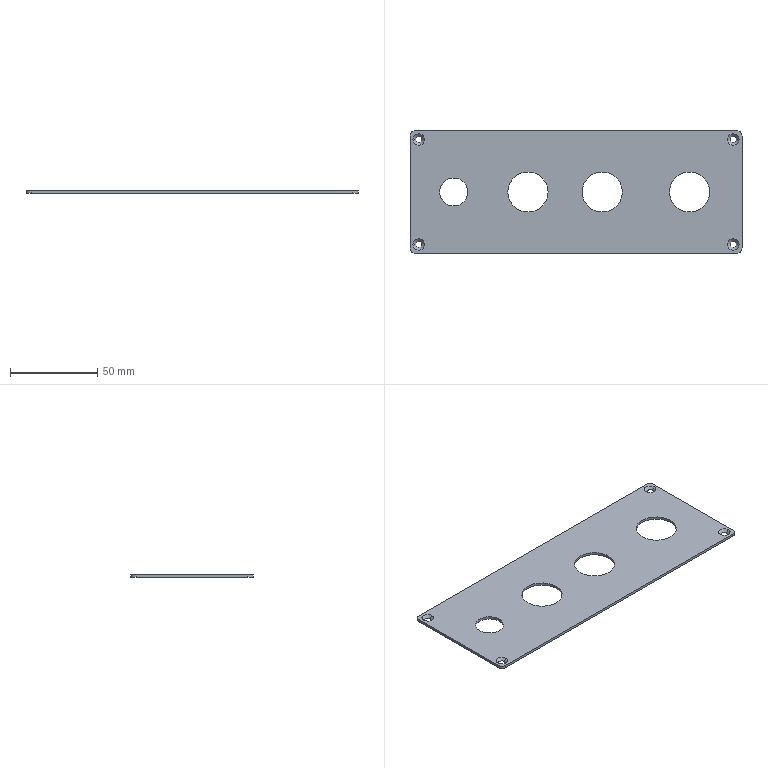Part | SolidWorks | features Extrusion 1, Fillet 1, HoleWzd 1, ICE 1 | 1 solid | 26 faces | box 190 x 70 x 1.5 mm | volume 17641 mm3 | cylinder 12 | cone 8 | plane 6 | commonest cylinder face diameters 23 x6 6 x4 16 x2
STEP:
#1=CARTESIAN_POINT('',(-91.8,30.,0.));
#2=VERTEX_POINT('',#1);
#3=CARTESIAN_POINT('',(-88.2,30.,0.));
#4=VERTEX_POINT('',#3);
#5=CARTESIAN_POINT('',(-90.,30.,0.));
#6=DIRECTION('',(0.,0.,1.));
#7=DIRECTION('',(1.,0.,0.));
#8=AXIS2_PLACEMENT_3D('',#5,#6,#7);
#9=CIRCLE('',#8,1.8);
#10=EDGE_CURVE('',#2,#4,#9,.T.);
#11=ORIENTED_EDGE('',*,*,#10,.F.);
#12=CARTESIAN_POINT('',(-93.3,30.,1.5));
#13=VERTEX_POINT('',#12);
#14=CARTESIAN_POINT('',(-93.3,30.,1.5));
#15=DIRECTION('',(-0.7071,0.,0.7071));
#16=VECTOR('',#15,1000.);
#17=LINE('',#14,#16);
#18=EDGE_CURVE('',#2,#13,#17,.T.);
#19=ORIENTED_EDGE('',*,*,#18,.T.);
#20=CARTESIAN_POINT('',(-86.7,30.,1.5));
#21=VERTEX_POINT('',#20);
#22=CARTESIAN_POINT('',(-90.,30.,1.5));
#23=DIRECTION('',(0.,0.,1.));
#24=DIRECTION('',(1.,0.,0.));
#25=AXIS2_PLACEMENT_3D('',#22,#23,#24);
#26=CIRCLE('',#25,3.3);
#27=EDGE_CURVE('',#13,#21,#26,.T.);
#28=ORIENTED_EDGE('',*,*,#27,.T.);
#29=CARTESIAN_POINT('',(-86.7,30.,1.5));
#30=DIRECTION('',(0.7071,0.,0.7071));
#31=VECTOR('',#30,1000.);
#32=LINE('',#29,#31);
#33=EDGE_CURVE('',#4,#21,#32,.T.);
#34=ORIENTED_EDGE('',*,*,#33,.F.);
#35=EDGE_LOOP('',(#11,#19,#28,#34));
#36=FACE_OUTER_BOUND('',#35,.T.);
#37=CARTESIAN_POINT('',(-90.,30.,1.5));
#38=DIRECTION('',(0.,0.,1.));
#39=DIRECTION('',(1.,0.,0.));
#40=AXIS2_PLACEMENT_3D('',#37,#38,#39);
#41=CONICAL_SURFACE('',#40,3.3,0.7854);
#42=ADVANCED_FACE('',(#36),#41,.F.);
#43=CARTESIAN_POINT('',(-91.8,-30.,0.));
#44=VERTEX_POINT('',#43);
#45=CARTESIAN_POINT('',(-88.2,-30.,0.));
#46=VERTEX_POINT('',#45);
#47=CARTESIAN_POINT('',(-90.,-30.,0.));
#48=DIRECTION('',(0.,0.,1.));
#49=DIRECTION('',(1.,0.,0.));
#50=AXIS2_PLACEMENT_3D('',#47,#48,#49);
#51=CIRCLE('',#50,1.8);
#52=EDGE_CURVE('',#44,#46,#51,.T.);
#53=ORIENTED_EDGE('',*,*,#52,.F.);
#54=CARTESIAN_POINT('',(-93.3,-30.,1.5));
#55=VERTEX_POINT('',#54);
#56=CARTESIAN_POINT('',(-93.3,-30.,1.5));
#57=DIRECTION('',(-0.7071,0.,0.7071));
#58=VECTOR('',#57,1000.);
#59=LINE('',#56,#58);
#60=EDGE_CURVE('',#44,#55,#59,.T.);
#61=ORIENTED_EDGE('',*,*,#60,.T.);
#62=CARTESIAN_POINT('',(-86.7,-30.,1.5));
#63=VERTEX_POINT('',#62);
#64=CARTESIAN_POINT('',(-90.,-30.,1.5));
#65=DIRECTION('',(0.,0.,1.));
#66=DIRECTION('',(1.,0.,0.));
#67=AXIS2_PLACEMENT_3D('',#64,#65,#66);
#68=CIRCLE('',#67,3.3);
#69=EDGE_CURVE('',#55,#63,#68,.T.);
#70=ORIENTED_EDGE('',*,*,#69,.T.);
#71=CARTESIAN_POINT('',(-86.7,-30.,1.5));
#72=DIRECTION('',(0.7071,0.,0.7071));
#73=VECTOR('',#72,1000.);
#74=LINE('',#71,#73);
#75=EDGE_CURVE('',#46,#63,#74,.T.);
#76=ORIENTED_EDGE('',*,*,#75,.F.);
#77=EDGE_LOOP('',(#53,#61,#70,#76));
#78=FACE_OUTER_BOUND('',#77,.T.);
#79=CARTESIAN_POINT('',(-90.,-30.,1.5));
#80=DIRECTION('',(0.,0.,1.));
#81=DIRECTION('',(1.,0.,0.));
#82=AXIS2_PLACEMENT_3D('',#79,#80,#81);
#83=CONICAL_SURFACE('',#82,3.3,0.7854);
#84=ADVANCED_FACE('',(#78),#83,.F.);
#85=CARTESIAN_POINT('',(88.2,-30.,0.));
#86=VERTEX_POINT('',#85);
#87=CARTESIAN_POINT('',(91.8,-30.,0.));
#88=VERTEX_POINT('',#87);
#89=CARTESIAN_POINT('',(90.,-30.,0.));
#90=DIRECTION('',(0.,0.,1.));
#91=DIRECTION('',(1.,0.,0.));
#92=AXIS2_PLACEMENT_3D('',#89,#90,#91);
#93=CIRCLE('',#92,1.8);
#94=EDGE_CURVE('',#86,#88,#93,.T.);
#95=ORIENTED_EDGE('',*,*,#94,.F.);
#96=CARTESIAN_POINT('',(86.7,-30.,1.5));
#97=VERTEX_POINT('',#96);
#98=CARTESIAN_POINT('',(86.7,-30.,1.5));
#99=DIRECTION('',(-0.7071,0.,0.7071));
#100=VECTOR('',#99,1000.);
#101=LINE('',#98,#100);
#102=EDGE_CURVE('',#86,#97,#101,.T.);
#103=ORIENTED_EDGE('',*,*,#102,.T.);
#104=CARTESIAN_POINT('',(93.3,-30.,1.5));
#105=VERTEX_POINT('',#104);
#106=CARTESIAN_POINT('',(90.,-30.,1.5));
#107=DIRECTION('',(0.,0.,1.));
#108=DIRECTION('',(1.,0.,0.));
#109=AXIS2_PLACEMENT_3D('',#106,#107,#108);
#110=CIRCLE('',#109,3.3);
#111=EDGE_CURVE('',#97,#105,#110,.T.);
#112=ORIENTED_EDGE('',*,*,#111,.T.);
#113=CARTESIAN_POINT('',(93.3,-30.,1.5));
#114=DIRECTION('',(0.7071,0.,0.7071));
#115=VECTOR('',#114,1000.);
#116=LINE('',#113,#115);
#117=EDGE_CURVE('',#88,#105,#116,.T.);
#118=ORIENTED_EDGE('',*,*,#117,.F.);
#119=EDGE_LOOP('',(#95,#103,#112,#118));
#120=FACE_OUTER_BOUND('',#119,.T.);
#121=CARTESIAN_POINT('',(90.,-30.,1.5));
#122=DIRECTION('',(0.,0.,1.));
#123=DIRECTION('',(1.,0.,0.));
#124=AXIS2_PLACEMENT_3D('',#121,#122,#123);
#125=CONICAL_SURFACE('',#124,3.3,0.7854);
#126=ADVANCED_FACE('',(#120),#125,.F.);
#127=CARTESIAN_POINT('',(88.2,30.,0.));
#128=VERTEX_POINT('',#127);
#129=CARTESIAN_POINT('',(91.8,30.,0.));
#130=VERTEX_POINT('',#129);
#131=CARTESIAN_POINT('',(90.,30.,0.));
#132=DIRECTION('',(0.,0.,1.));
#133=DIRECTION('',(1.,0.,0.));
#134=AXIS2_PLACEMENT_3D('',#131,#132,#133);
#135=CIRCLE('',#134,1.8);
#136=EDGE_CURVE('',#128,#130,#135,.T.);
#137=ORIENTED_EDGE('',*,*,#136,.F.);
#138=CARTESIAN_POINT('',(86.7,30.,1.5));
#139=VERTEX_POINT('',#138);
#140=CARTESIAN_POINT('',(86.7,30.,1.5));
#141=DIRECTION('',(-0.7071,0.,0.7071));
#142=VECTOR('',#141,1000.);
#143=LINE('',#140,#142);
#144=EDGE_CURVE('',#128,#139,#143,.T.);
#145=ORIENTED_EDGE('',*,*,#144,.T.);
#146=CARTESIAN_POINT('',(93.3,30.,1.5));
#147=VERTEX_POINT('',#146);
#148=CARTESIAN_POINT('',(90.,30.,1.5));
#149=DIRECTION('',(0.,0.,1.));
#150=DIRECTION('',(1.,0.,0.));
#151=AXIS2_PLACEMENT_3D('',#148,#149,#150);
#152=CIRCLE('',#151,3.3);
#153=EDGE_CURVE('',#139,#147,#152,.T.);
#154=ORIENTED_EDGE('',*,*,#153,.T.);
#155=CARTESIAN_POINT('',(93.3,30.,1.5));
#156=DIRECTION('',(0.7071,0.,0.7071));
#157=VECTOR('',#156,1000.);
#158=LINE('',#155,#157);
#159=EDGE_CURVE('',#130,#147,#158,.T.);
#160=ORIENTED_EDGE('',*,*,#159,.F.);
#161=EDGE_LOOP('',(#137,#145,#154,#160));
#162=FACE_OUTER_BOUND('',#161,.T.);
#163=CARTESIAN_POINT('',(90.,30.,1.5));
#164=DIRECTION('',(0.,0.,1.));
#165=DIRECTION('',(1.,0.,0.));
#166=AXIS2_PLACEMENT_3D('',#163,#164,#165);
#167=CONICAL_SURFACE('',#166,3.3,0.7854);
#168=ADVANCED_FACE('',(#162),#167,.F.);
#169=CARTESIAN_POINT('',(53.5,0.,0.));
#170=VERTEX_POINT('',#169);
#171=CARTESIAN_POINT('',(76.5,0.,0.));
#172=VERTEX_POINT('',#171);
#173=CARTESIAN_POINT('',(65.,0.,0.));
#174=DIRECTION('',(0.,0.,1.));
#175=DIRECTION('',(1.,0.,0.));
#176=AXIS2_PLACEMENT_3D('',#173,#174,#175);
#177=CIRCLE('',#176,11.5);
#178=EDGE_CURVE('',#170,#172,#177,.T.);
#179=ORIENTED_EDGE('',*,*,#178,.F.);
#180=CARTESIAN_POINT('',(53.5,0.,1.5));
#181=VERTEX_POINT('',#180);
#182=CARTESIAN_POINT('',(53.5,0.,0.));
#183=DIRECTION('',(0.,0.,1.));
#184=VECTOR('',#183,1000.);
#185=LINE('',#182,#184);
#186=EDGE_CURVE('',#170,#181,#185,.T.);
#187=ORIENTED_EDGE('',*,*,#186,.T.);
#188=CARTESIAN_POINT('',(76.5,0.,1.5));
#189=VERTEX_POINT('',#188);
#190=CARTESIAN_POINT('',(65.,0.,1.5));
#191=DIRECTION('',(0.,0.,1.));
#192=DIRECTION('',(1.,0.,0.));
#193=AXIS2_PLACEMENT_3D('',#190,#191,#192);
#194=CIRCLE('',#193,11.5);
#195=EDGE_CURVE('',#181,#189,#194,.T.);
#196=ORIENTED_EDGE('',*,*,#195,.T.);
#197=CARTESIAN_POINT('',(76.5,0.,0.));
#198=DIRECTION('',(0.,0.,1.));
#199=VECTOR('',#198,1000.);
#200=LINE('',#197,#199);
#201=EDGE_CURVE('',#172,#189,#200,.T.);
#202=ORIENTED_EDGE('',*,*,#201,.F.);
#203=EDGE_LOOP('',(#179,#187,#196,#202));
#204=FACE_OUTER_BOUND('',#203,.T.);
#205=CARTESIAN_POINT('',(65.,0.,0.));
#206=DIRECTION('',(0.,0.,1.));
#207=DIRECTION('',(1.,0.,0.));
#208=AXIS2_PLACEMENT_3D('',#205,#206,#207);
#209=CYLINDRICAL_SURFACE('',#208,11.5);
#210=ADVANCED_FACE('',(#204),#209,.F.);
#211=CARTESIAN_POINT('',(-78.,0.,0.));
#212=VERTEX_POINT('',#211);
#213=CARTESIAN_POINT('',(-62.,0.,0.));
#214=VERTEX_POINT('',#213);
#215=CARTESIAN_POINT('',(-70.,0.,0.));
#216=DIRECTION('',(0.,0.,1.));
#217=DIRECTION('',(1.,0.,0.));
#218=AXIS2_PLACEMENT_3D('',#215,#216,#217);
#219=CIRCLE('',#218,8.);
#220=EDGE_CURVE('',#212,#214,#219,.T.);
#221=ORIENTED_EDGE('',*,*,#220,.F.);
#222=CARTESIAN_POINT('',(-78.,0.,1.5));
#223=VERTEX_POINT('',#222);
#224=CARTESIAN_POINT('',(-78.,0.,0.));
#225=DIRECTION('',(0.,0.,1.));
#226=VECTOR('',#225,1000.);
#227=LINE('',#224,#226);
#228=EDGE_CURVE('',#212,#223,#227,.T.);
#229=ORIENTED_EDGE('',*,*,#228,.T.);
#230=CARTESIAN_POINT('',(-62.,0.,1.5));
#231=VERTEX_POINT('',#230);
#232=CARTESIAN_POINT('',(-70.,0.,1.5));
#233=DIRECTION('',(0.,0.,1.));
#234=DIRECTION('',(1.,0.,0.));
#235=AXIS2_PLACEMENT_3D('',#232,#233,#234);
#236=CIRCLE('',#235,8.);
#237=EDGE_CURVE('',#223,#231,#236,.T.);
#238=ORIENTED_EDGE('',*,*,#237,.T.);
#239=CARTESIAN_POINT('',(-62.,0.,0.));
#240=DIRECTION('',(0.,0.,1.));
#241=VECTOR('',#240,1000.);
#242=LINE('',#239,#241);
#243=EDGE_CURVE('',#214,#231,#242,.T.);
#244=ORIENTED_EDGE('',*,*,#243,.F.);
#245=EDGE_LOOP('',(#221,#229,#238,#244));
#246=FACE_OUTER_BOUND('',#245,.T.);
#247=CARTESIAN_POINT('',(-70.,0.,0.));
#248=DIRECTION('',(0.,0.,1.));
#249=DIRECTION('',(1.,0.,0.));
#250=AXIS2_PLACEMENT_3D('',#247,#248,#249);
#251=CYLINDRICAL_SURFACE('',#250,8.);
#252=ADVANCED_FACE('',(#246),#251,.F.);
#253=CARTESIAN_POINT('',(-39.,0.,0.));
#254=VERTEX_POINT('',#253);
#255=CARTESIAN_POINT('',(-16.,0.,0.));
#256=VERTEX_POINT('',#255);
#257=CARTESIAN_POINT('',(-27.5,0.,0.));
#258=DIRECTION('',(0.,0.,1.));
#259=DIRECTION('',(1.,0.,0.));
#260=AXIS2_PLACEMENT_3D('',#257,#258,#259);
#261=CIRCLE('',#260,11.5);
#262=EDGE_CURVE('',#254,#256,#261,.T.);
#263=ORIENTED_EDGE('',*,*,#262,.F.);
#264=CARTESIAN_POINT('',(-39.,0.,1.5));
#265=VERTEX_POINT('',#264);
#266=CARTESIAN_POINT('',(-39.,0.,0.));
#267=DIRECTION('',(0.,0.,1.));
#268=VECTOR('',#267,1000.);
#269=LINE('',#266,#268);
#270=EDGE_CURVE('',#254,#265,#269,.T.);
#271=ORIENTED_EDGE('',*,*,#270,.T.);
#272=CARTESIAN_POINT('',(-16.,0.,1.5));
#273=VERTEX_POINT('',#272);
#274=CARTESIAN_POINT('',(-27.5,0.,1.5));
#275=DIRECTION('',(0.,0.,1.));
#276=DIRECTION('',(1.,0.,0.));
#277=AXIS2_PLACEMENT_3D('',#274,#275,#276);
#278=CIRCLE('',#277,11.5);
#279=EDGE_CURVE('',#265,#273,#278,.T.);
#280=ORIENTED_EDGE('',*,*,#279,.T.);
#281=CARTESIAN_POINT('',(-16.,0.,0.));
#282=DIRECTION('',(0.,0.,1.));
#283=VECTOR('',#282,1000.);
#284=LINE('',#281,#283);
#285=EDGE_CURVE('',#256,#273,#284,.T.);
#286=ORIENTED_EDGE('',*,*,#285,.F.);
#287=EDGE_LOOP('',(#263,#271,#280,#286));
#288=FACE_OUTER_BOUND('',#287,.T.);
#289=CARTESIAN_POINT('',(-27.5,0.,0.));
#290=DIRECTION('',(0.,0.,1.));
#291=DIRECTION('',(1.,0.,0.));
#292=AXIS2_PLACEMENT_3D('',#289,#290,#291);
#293=CYLINDRICAL_SURFACE('',#292,11.5);
#294=ADVANCED_FACE('',(#288),#293,.F.);
#295=CARTESIAN_POINT('',(3.5,0.,0.));
#296=VERTEX_POINT('',#295);
#297=CARTESIAN_POINT('',(26.5,0.,0.));
#298=VERTEX_POINT('',#297);
#299=CARTESIAN_POINT('',(15.,0.,0.));
#300=DIRECTION('',(0.,0.,1.));
#301=DIRECTION('',(1.,0.,0.));
#302=AXIS2_PLACEMENT_3D('',#299,#300,#301);
#303=CIRCLE('',#302,11.5);
#304=EDGE_CURVE('',#296,#298,#303,.T.);
#305=ORIENTED_EDGE('',*,*,#304,.F.);
#306=CARTESIAN_POINT('',(3.5,0.,1.5));
#307=VERTEX_POINT('',#306);
#308=CARTESIAN_POINT('',(3.5,0.,0.));
#309=DIRECTION('',(0.,0.,1.));
#310=VECTOR('',#309,1000.);
#311=LINE('',#308,#310);
#312=EDGE_CURVE('',#296,#307,#311,.T.);
#313=ORIENTED_EDGE('',*,*,#312,.T.);
#314=CARTESIAN_POINT('',(26.5,0.,1.5));
#315=VERTEX_POINT('',#314);
#316=CARTESIAN_POINT('',(15.,0.,1.5));
#317=DIRECTION('',(0.,0.,1.));
#318=DIRECTION('',(1.,0.,0.));
#319=AXIS2_PLACEMENT_3D('',#316,#317,#318);
#320=CIRCLE('',#319,11.5);
#321=EDGE_CURVE('',#307,#315,#320,.T.);
#322=ORIENTED_EDGE('',*,*,#321,.T.);
#323=CARTESIAN_POINT('',(26.5,0.,0.));
#324=DIRECTION('',(0.,0.,1.));
#325=VECTOR('',#324,1000.);
#326=LINE('',#323,#325);
#327=EDGE_CURVE('',#298,#315,#326,.T.);
#328=ORIENTED_EDGE('',*,*,#327,.F.);
#329=EDGE_LOOP('',(#305,#313,#322,#328));
#330=FACE_OUTER_BOUND('',#329,.T.);
#331=CARTESIAN_POINT('',(15.,0.,0.));
#332=DIRECTION('',(0.,0.,1.));
#333=DIRECTION('',(1.,0.,0.));
#334=AXIS2_PLACEMENT_3D('',#331,#332,#333);
#335=CYLINDRICAL_SURFACE('',#334,11.5);
#336=ADVANCED_FACE('',(#330),#335,.F.);
#337=CARTESIAN_POINT('',(-90.,30.,0.));
#338=DIRECTION('',(0.,0.,1.));
#339=DIRECTION('',(1.,0.,0.));
#340=AXIS2_PLACEMENT_3D('',#337,#338,#339);
#341=CIRCLE('',#340,1.8);
#342=EDGE_CURVE('',#4,#2,#341,.T.);
#343=ORIENTED_EDGE('',*,*,#342,.T.);
#344=ORIENTED_EDGE('',*,*,#10,.T.);
#345=EDGE_LOOP('',(#343,#344));
#346=FACE_BOUND('',#345,.T.);
#347=CARTESIAN_POINT('',(-90.,-30.,0.));
#348=DIRECTION('',(0.,0.,1.));
#349=DIRECTION('',(1.,0.,0.));
#350=AXIS2_PLACEMENT_3D('',#347,#348,#349);
#351=CIRCLE('',#350,1.8);
#352=EDGE_CURVE('',#46,#44,#351,.T.);
#353=ORIENTED_EDGE('',*,*,#352,.T.);
#354=ORIENTED_EDGE('',*,*,#52,.T.);
#355=EDGE_LOOP('',(#353,#354));
#356=FACE_BOUND('',#355,.T.);
#357=CARTESIAN_POINT('',(90.,-30.,0.));
#358=DIRECTION('',(0.,0.,1.));
#359=DIRECTION('',(1.,0.,0.));
#360=AXIS2_PLACEMENT_3D('',#357,#358,#359);
#361=CIRCLE('',#360,1.8);
#362=EDGE_CURVE('',#88,#86,#361,.T.);
#363=ORIENTED_EDGE('',*,*,#362,.T.);
#364=ORIENTED_EDGE('',*,*,#94,.T.);
#365=EDGE_LOOP('',(#363,#364));
#366=FACE_BOUND('',#365,.T.);
#367=CARTESIAN_POINT('',(90.,30.,0.));
#368=DIRECTION('',(0.,0.,1.));
#369=DIRECTION('',(1.,0.,0.));
#370=AXIS2_PLACEMENT_3D('',#367,#368,#369);
#371=CIRCLE('',#370,1.8);
#372=EDGE_CURVE('',#130,#128,#371,.T.);
#373=ORIENTED_EDGE('',*,*,#372,.T.);
#374=ORIENTED_EDGE('',*,*,#136,.T.);
#375=EDGE_LOOP('',(#373,#374));
#376=FACE_BOUND('',#375,.T.);
#377=CARTESIAN_POINT('',(65.,0.,0.));
#378=DIRECTION('',(0.,0.,1.));
#379=DIRECTION('',(1.,0.,0.));
#380=AXIS2_PLACEMENT_3D('',#377,#378,#379);
#381=CIRCLE('',#380,11.5);
#382=EDGE_CURVE('',#172,#170,#381,.T.);
#383=ORIENTED_EDGE('',*,*,#382,.T.);
#384=ORIENTED_EDGE('',*,*,#178,.T.);
#385=EDGE_LOOP('',(#383,#384));
#386=FACE_BOUND('',#385,.T.);
#387=CARTESIAN_POINT('',(-70.,0.,0.));
#388=DIRECTION('',(0.,0.,1.));
#389=DIRECTION('',(1.,0.,0.));
#390=AXIS2_PLACEMENT_3D('',#387,#388,#389);
#391=CIRCLE('',#390,8.);
#392=EDGE_CURVE('',#214,#212,#391,.T.);
#393=ORIENTED_EDGE('',*,*,#392,.T.);
#394=ORIENTED_EDGE('',*,*,#220,.T.);
#395=EDGE_LOOP('',(#393,#394));
#396=FACE_BOUND('',#395,.T.);
#397=CARTESIAN_POINT('',(-27.5,0.,0.));
#398=DIRECTION('',(0.,0.,1.));
#399=DIRECTION('',(1.,0.,0.));
#400=AXIS2_PLACEMENT_3D('',#397,#398,#399);
#401=CIRCLE('',#400,11.5);
#402=EDGE_CURVE('',#256,#254,#401,.T.);
#403=ORIENTED_EDGE('',*,*,#402,.T.);
#404=ORIENTED_EDGE('',*,*,#262,.T.);
#405=EDGE_LOOP('',(#403,#404));
#406=FACE_BOUND('',#405,.T.);
#407=CARTESIAN_POINT('',(15.,0.,0.));
#408=DIRECTION('',(0.,0.,1.));
#409=DIRECTION('',(1.,0.,0.));
#410=AXIS2_PLACEMENT_3D('',#407,#408,#409);
#411=CIRCLE('',#410,11.5);
#412=EDGE_CURVE('',#298,#296,#411,.T.);
#413=ORIENTED_EDGE('',*,*,#412,.T.);
#414=ORIENTED_EDGE('',*,*,#304,.T.);
#415=EDGE_LOOP('',(#413,#414));
#416=FACE_BOUND('',#415,.T.);
#417=CARTESIAN_POINT('',(-95.,32.,0.));
#418=VERTEX_POINT('',#417);
#419=CARTESIAN_POINT('',(-95.,-32.,0.));
#420=VERTEX_POINT('',#419);
#421=CARTESIAN_POINT('',(-95.,35.,0.));
#422=DIRECTION('',(0.,-1.,0.));
#423=VECTOR('',#422,1000.);
#424=LINE('',#421,#423);
#425=EDGE_CURVE('',#418,#420,#424,.T.);
#426=ORIENTED_EDGE('',*,*,#425,.F.);
#427=CARTESIAN_POINT('',(-92.,35.,0.));
#428=VERTEX_POINT('',#427);
#429=CARTESIAN_POINT('',(-92.,32.,0.));
#430=DIRECTION('',(0.,0.,-1.));
#431=DIRECTION('',(1.,0.,0.));
#432=AXIS2_PLACEMENT_3D('',#429,#430,#431);
#433=CIRCLE('',#432,3.);
#434=EDGE_CURVE('',#418,#428,#433,.T.);
#435=ORIENTED_EDGE('',*,*,#434,.T.);
#436=CARTESIAN_POINT('',(92.,35.,0.));
#437=VERTEX_POINT('',#436);
#438=CARTESIAN_POINT('',(-95.,35.,0.));
#439=DIRECTION('',(-1.,0.,0.));
#440=VECTOR('',#439,1000.);
#441=LINE('',#438,#440);
#442=EDGE_CURVE('',#437,#428,#441,.T.);
#443=ORIENTED_EDGE('',*,*,#442,.F.);
#444=CARTESIAN_POINT('',(95.,32.,0.));
#445=VERTEX_POINT('',#444);
#446=CARTESIAN_POINT('',(92.,32.,0.));
#447=DIRECTION('',(0.,0.,-1.));
#448=DIRECTION('',(1.,0.,0.));
#449=AXIS2_PLACEMENT_3D('',#446,#447,#448);
#450=CIRCLE('',#449,3.);
#451=EDGE_CURVE('',#437,#445,#450,.T.);
#452=ORIENTED_EDGE('',*,*,#451,.T.);
#453=CARTESIAN_POINT('',(95.,-32.,0.));
#454=VERTEX_POINT('',#453);
#455=CARTESIAN_POINT('',(95.,35.,0.));
#456=DIRECTION('',(0.,1.,0.));
#457=VECTOR('',#456,1000.);
#458=LINE('',#455,#457);
#459=EDGE_CURVE('',#454,#445,#458,.T.);
#460=ORIENTED_EDGE('',*,*,#459,.F.);
#461=CARTESIAN_POINT('',(92.,-35.,0.));
#462=VERTEX_POINT('',#461);
#463=CARTESIAN_POINT('',(92.,-32.,0.));
#464=DIRECTION('',(0.,0.,-1.));
#465=DIRECTION('',(1.,0.,0.));
#466=AXIS2_PLACEMENT_3D('',#463,#464,#465);
#467=CIRCLE('',#466,3.);
#468=EDGE_CURVE('',#454,#462,#467,.T.);
#469=ORIENTED_EDGE('',*,*,#468,.T.);
#470=CARTESIAN_POINT('',(-92.,-35.,0.));
#471=VERTEX_POINT('',#470);
#472=CARTESIAN_POINT('',(-95.,-35.,0.));
#473=DIRECTION('',(1.,0.,0.));
#474=VECTOR('',#473,1000.);
#475=LINE('',#472,#474);
#476=EDGE_CURVE('',#471,#462,#475,.T.);
#477=ORIENTED_EDGE('',*,*,#476,.F.);
#478=CARTESIAN_POINT('',(-92.,-32.,0.));
#479=DIRECTION('',(0.,0.,-1.));
#480=DIRECTION('',(1.,0.,0.));
#481=AXIS2_PLACEMENT_3D('',#478,#479,#480);
#482=CIRCLE('',#481,3.);
#483=EDGE_CURVE('',#471,#420,#482,.T.);
#484=ORIENTED_EDGE('',*,*,#483,.T.);
#485=EDGE_LOOP('',(#426,#435,#443,#452,#460,#469,#477,#484));
#486=FACE_OUTER_BOUND('',#485,.T.);
#487=CARTESIAN_POINT('',(95.,-35.,0.));
#488=DIRECTION('',(0.,0.,1.));
#489=DIRECTION('',(1.,0.,0.));
#490=AXIS2_PLACEMENT_3D('',#487,#488,#489);
#491=PLANE('',#490);
#492=ADVANCED_FACE('',(#346,#356,#366,#376,#386,#396,#406,#416,#486),#491,.F.);
#493=CARTESIAN_POINT('',(95.,-32.,1.5));
#494=VERTEX_POINT('',#493);
#495=CARTESIAN_POINT('',(95.,32.,1.5));
#496=VERTEX_POINT('',#495);
#497=CARTESIAN_POINT('',(95.,35.,1.5));
#498=DIRECTION('',(0.,1.,0.));
#499=VECTOR('',#498,1000.);
#500=LINE('',#497,#499);
#501=EDGE_CURVE('',#494,#496,#500,.T.);
#502=ORIENTED_EDGE('',*,*,#501,.F.);
#503=CARTESIAN_POINT('',(95.,-32.,1.5));
#504=DIRECTION('',(0.,0.,-1.));
#505=VECTOR('',#504,1000.);
#506=LINE('',#503,#505);
#507=EDGE_CURVE('',#494,#454,#506,.T.);
#508=ORIENTED_EDGE('',*,*,#507,.T.);
#509=ORIENTED_EDGE('',*,*,#459,.T.);
#510=CARTESIAN_POINT('',(95.,32.,1.5));
#511=DIRECTION('',(0.,0.,1.));
#512=VECTOR('',#511,1000.);
#513=LINE('',#510,#512);
#514=EDGE_CURVE('',#445,#496,#513,.T.);
#515=ORIENTED_EDGE('',*,*,#514,.T.);
#516=EDGE_LOOP('',(#502,#508,#509,#515));
#517=FACE_OUTER_BOUND('',#516,.T.);
#518=CARTESIAN_POINT('',(95.,35.,1.5));
#519=DIRECTION('',(-1.,0.,0.));
#520=DIRECTION('',(0.,0.,1.));
#521=AXIS2_PLACEMENT_3D('',#518,#519,#520);
#522=PLANE('',#521);
#523=ADVANCED_FACE('',(#517),#522,.F.);
#524=ORIENTED_EDGE('',*,*,#442,.T.);
#525=CARTESIAN_POINT('',(-92.,35.,1.5));
#526=VERTEX_POINT('',#525);
#527=CARTESIAN_POINT('',(-92.,35.,1.5));
#528=DIRECTION('',(0.,0.,1.));
#529=VECTOR('',#528,1000.);
#530=LINE('',#527,#529);
#531=EDGE_CURVE('',#428,#526,#530,.T.);
#532=ORIENTED_EDGE('',*,*,#531,.T.);
#533=CARTESIAN_POINT('',(92.,35.,1.5));
#534=VERTEX_POINT('',#533);
#535=CARTESIAN_POINT('',(-95.,35.,1.5));
#536=DIRECTION('',(-1.,0.,0.));
#537=VECTOR('',#536,1000.);
#538=LINE('',#535,#537);
#539=EDGE_CURVE('',#534,#526,#538,.T.);
#540=ORIENTED_EDGE('',*,*,#539,.F.);
#541=CARTESIAN_POINT('',(92.,35.,1.5));
#542=DIRECTION('',(0.,0.,-1.));
#543=VECTOR('',#542,1000.);
#544=LINE('',#541,#543);
#545=EDGE_CURVE('',#534,#437,#544,.T.);
#546=ORIENTED_EDGE('',*,*,#545,.T.);
#547=EDGE_LOOP('',(#524,#532,#540,#546));
#548=FACE_OUTER_BOUND('',#547,.T.);
#549=CARTESIAN_POINT('',(-95.,35.,1.5));
#550=DIRECTION('',(0.,-1.,0.));
#551=DIRECTION('',(0.,0.,-1.));
#552=AXIS2_PLACEMENT_3D('',#549,#550,#551);
#553=PLANE('',#552);
#554=ADVANCED_FACE('',(#548),#553,.F.);
#555=CARTESIAN_POINT('',(-95.,32.,1.5));
#556=VERTEX_POINT('',#555);
#557=CARTESIAN_POINT('',(-95.,-32.,1.5));
#558=VERTEX_POINT('',#557);
#559=CARTESIAN_POINT('',(-95.,35.,1.5));
#560=DIRECTION('',(0.,-1.,0.));
#561=VECTOR('',#560,1000.);
#562=LINE('',#559,#561);
#563=EDGE_CURVE('',#556,#558,#562,.T.);
#564=ORIENTED_EDGE('',*,*,#563,.F.);
#565=CARTESIAN_POINT('',(-95.,32.,1.5));
#566=DIRECTION('',(0.,0.,-1.));
#567=VECTOR('',#566,1000.);
#568=LINE('',#565,#567);
#569=EDGE_CURVE('',#556,#418,#568,.T.);
#570=ORIENTED_EDGE('',*,*,#569,.T.);
#571=ORIENTED_EDGE('',*,*,#425,.T.);
#572=CARTESIAN_POINT('',(-95.,-32.,1.5));
#573=DIRECTION('',(0.,0.,1.));
#574=VECTOR('',#573,1000.);
#575=LINE('',#572,#574);
#576=EDGE_CURVE('',#420,#558,#575,.T.);
#577=ORIENTED_EDGE('',*,*,#576,.T.);
#578=EDGE_LOOP('',(#564,#570,#571,#577));
#579=FACE_OUTER_BOUND('',#578,.T.);
#580=CARTESIAN_POINT('',(-95.,35.,1.5));
#581=DIRECTION('',(1.,0.,0.));
#582=DIRECTION('',(0.,0.,-1.));
#583=AXIS2_PLACEMENT_3D('',#580,#581,#582);
#584=PLANE('',#583);
#585=ADVANCED_FACE('',(#579),#584,.F.);
#586=CARTESIAN_POINT('',(-92.,-35.,1.5));
#587=VERTEX_POINT('',#586);
#588=CARTESIAN_POINT('',(92.,-35.,1.5));
#589=VERTEX_POINT('',#588);
#590=CARTESIAN_POINT('',(-95.,-35.,1.5));
#591=DIRECTION('',(1.,0.,0.));
#592=VECTOR('',#591,1000.);
#593=LINE('',#590,#592);
#594=EDGE_CURVE('',#587,#589,#593,.T.);
#595=ORIENTED_EDGE('',*,*,#594,.F.);
#596=CARTESIAN_POINT('',(-92.,-35.,1.5));
#597=DIRECTION('',(0.,0.,-1.));
#598=VECTOR('',#597,1000.);
#599=LINE('',#596,#598);
#600=EDGE_CURVE('',#587,#471,#599,.T.);
#601=ORIENTED_EDGE('',*,*,#600,.T.);
#602=ORIENTED_EDGE('',*,*,#476,.T.);
#603=CARTESIAN_POINT('',(92.,-35.,1.5));
#604=DIRECTION('',(0.,0.,1.));
#605=VECTOR('',#604,1000.);
#606=LINE('',#603,#605);
#607=EDGE_CURVE('',#462,#589,#606,.T.);
#608=ORIENTED_EDGE('',*,*,#607,.T.);
#609=EDGE_LOOP('',(#595,#601,#602,#608));
#610=FACE_OUTER_BOUND('',#609,.T.);
#611=CARTESIAN_POINT('',(-95.,-35.,1.5));
#612=DIRECTION('',(0.,1.,0.));
#613=DIRECTION('',(0.,0.,1.));
#614=AXIS2_PLACEMENT_3D('',#611,#612,#613);
#615=PLANE('',#614);
#616=ADVANCED_FACE('',(#610),#615,.F.);
#617=CARTESIAN_POINT('',(-90.,30.,1.5));
#618=DIRECTION('',(0.,0.,1.));
#619=DIRECTION('',(1.,0.,0.));
#620=AXIS2_PLACEMENT_3D('',#617,#618,#619);
#621=CIRCLE('',#620,3.3);
#622=EDGE_CURVE('',#21,#13,#621,.T.);
#623=ORIENTED_EDGE('',*,*,#622,.F.);
#624=ORIENTED_EDGE('',*,*,#27,.F.);
#625=EDGE_LOOP('',(#623,#624));
#626=FACE_BOUND('',#625,.T.);
#627=CARTESIAN_POINT('',(-90.,-30.,1.5));
#628=DIRECTION('',(0.,0.,1.));
#629=DIRECTION('',(1.,0.,0.));
#630=AXIS2_PLACEMENT_3D('',#627,#628,#629);
#631=CIRCLE('',#630,3.3);
#632=EDGE_CURVE('',#63,#55,#631,.T.);
#633=ORIENTED_EDGE('',*,*,#632,.F.);
#634=ORIENTED_EDGE('',*,*,#69,.F.);
#635=EDGE_LOOP('',(#633,#634));
#636=FACE_BOUND('',#635,.T.);
#637=CARTESIAN_POINT('',(90.,-30.,1.5));
#638=DIRECTION('',(0.,0.,1.));
#639=DIRECTION('',(1.,0.,0.));
#640=AXIS2_PLACEMENT_3D('',#637,#638,#639);
#641=CIRCLE('',#640,3.3);
#642=EDGE_CURVE('',#105,#97,#641,.T.);
#643=ORIENTED_EDGE('',*,*,#642,.F.);
#644=ORIENTED_EDGE('',*,*,#111,.F.);
#645=EDGE_LOOP('',(#643,#644));
#646=FACE_BOUND('',#645,.T.);
#647=CARTESIAN_POINT('',(90.,30.,1.5));
#648=DIRECTION('',(0.,0.,1.));
#649=DIRECTION('',(1.,0.,0.));
#650=AXIS2_PLACEMENT_3D('',#647,#648,#649);
#651=CIRCLE('',#650,3.3);
#652=EDGE_CURVE('',#147,#139,#651,.T.);
#653=ORIENTED_EDGE('',*,*,#652,.F.);
#654=ORIENTED_EDGE('',*,*,#153,.F.);
#655=EDGE_LOOP('',(#653,#654));
#656=FACE_BOUND('',#655,.T.);
#657=CARTESIAN_POINT('',(65.,0.,1.5));
#658=DIRECTION('',(0.,0.,1.));
#659=DIRECTION('',(1.,0.,0.));
#660=AXIS2_PLACEMENT_3D('',#657,#658,#659);
#661=CIRCLE('',#660,11.5);
#662=EDGE_CURVE('',#189,#181,#661,.T.);
#663=ORIENTED_EDGE('',*,*,#662,.F.);
#664=ORIENTED_EDGE('',*,*,#195,.F.);
#665=EDGE_LOOP('',(#663,#664));
#666=FACE_BOUND('',#665,.T.);
#667=CARTESIAN_POINT('',(-70.,0.,1.5));
#668=DIRECTION('',(0.,0.,1.));
#669=DIRECTION('',(1.,0.,0.));
#670=AXIS2_PLACEMENT_3D('',#667,#668,#669);
#671=CIRCLE('',#670,8.);
#672=EDGE_CURVE('',#231,#223,#671,.T.);
#673=ORIENTED_EDGE('',*,*,#672,.F.);
#674=ORIENTED_EDGE('',*,*,#237,.F.);
#675=EDGE_LOOP('',(#673,#674));
#676=FACE_BOUND('',#675,.T.);
#677=CARTESIAN_POINT('',(-27.5,0.,1.5));
#678=DIRECTION('',(0.,0.,1.));
#679=DIRECTION('',(1.,0.,0.));
#680=AXIS2_PLACEMENT_3D('',#677,#678,#679);
#681=CIRCLE('',#680,11.5);
#682=EDGE_CURVE('',#273,#265,#681,.T.);
#683=ORIENTED_EDGE('',*,*,#682,.F.);
#684=ORIENTED_EDGE('',*,*,#279,.F.);
#685=EDGE_LOOP('',(#683,#684));
#686=FACE_BOUND('',#685,.T.);
#687=CARTESIAN_POINT('',(15.,0.,1.5));
#688=DIRECTION('',(0.,0.,1.));
#689=DIRECTION('',(1.,0.,0.));
#690=AXIS2_PLACEMENT_3D('',#687,#688,#689);
#691=CIRCLE('',#690,11.5);
#692=EDGE_CURVE('',#315,#307,#691,.T.);
#693=ORIENTED_EDGE('',*,*,#692,.F.);
#694=ORIENTED_EDGE('',*,*,#321,.F.);
#695=EDGE_LOOP('',(#693,#694));
#696=FACE_BOUND('',#695,.T.);
#697=ORIENTED_EDGE('',*,*,#539,.T.);
#698=CARTESIAN_POINT('',(-92.,32.,1.5));
#699=DIRECTION('',(0.,0.,1.));
#700=DIRECTION('',(1.,0.,0.));
#701=AXIS2_PLACEMENT_3D('',#698,#699,#700);
#702=CIRCLE('',#701,3.);
#703=EDGE_CURVE('',#526,#556,#702,.T.);
#704=ORIENTED_EDGE('',*,*,#703,.T.);
#705=ORIENTED_EDGE('',*,*,#563,.T.);
#706=CARTESIAN_POINT('',(-92.,-32.,1.5));
#707=DIRECTION('',(0.,0.,1.));
#708=DIRECTION('',(1.,0.,0.));
#709=AXIS2_PLACEMENT_3D('',#706,#707,#708);
#710=CIRCLE('',#709,3.);
#711=EDGE_CURVE('',#558,#587,#710,.T.);
#712=ORIENTED_EDGE('',*,*,#711,.T.);
#713=ORIENTED_EDGE('',*,*,#594,.T.);
#714=CARTESIAN_POINT('',(92.,-32.,1.5));
#715=DIRECTION('',(0.,0.,1.));
#716=DIRECTION('',(1.,0.,0.));
#717=AXIS2_PLACEMENT_3D('',#714,#715,#716);
#718=CIRCLE('',#717,3.);
#719=EDGE_CURVE('',#589,#494,#718,.T.);
#720=ORIENTED_EDGE('',*,*,#719,.T.);
#721=ORIENTED_EDGE('',*,*,#501,.T.);
#722=CARTESIAN_POINT('',(92.,32.,1.5));
#723=DIRECTION('',(0.,0.,1.));
#724=DIRECTION('',(1.,0.,0.));
#725=AXIS2_PLACEMENT_3D('',#722,#723,#724);
#726=CIRCLE('',#725,3.);
#727=EDGE_CURVE('',#496,#534,#726,.T.);
#728=ORIENTED_EDGE('',*,*,#727,.T.);
#729=EDGE_LOOP('',(#697,#704,#705,#712,#713,#720,#721,#728));
#730=FACE_OUTER_BOUND('',#729,.T.);
#731=CARTESIAN_POINT('',(95.,-35.,1.5));
#732=DIRECTION('',(0.,0.,1.));
#733=DIRECTION('',(1.,0.,0.));
#734=AXIS2_PLACEMENT_3D('',#731,#732,#733);
#735=PLANE('',#734);
#736=ADVANCED_FACE('',(#626,#636,#646,#656,#666,#676,#686,#696,#730),#735,.T.);
#737=ORIENTED_EDGE('',*,*,#703,.F.);
#738=ORIENTED_EDGE('',*,*,#531,.F.);
#739=ORIENTED_EDGE('',*,*,#434,.F.);
#740=ORIENTED_EDGE('',*,*,#569,.F.);
#741=EDGE_LOOP('',(#737,#738,#739,#740));
#742=FACE_OUTER_BOUND('',#741,.T.);
#743=CARTESIAN_POINT('',(-92.,32.,1.5));
#744=DIRECTION('',(0.,0.,-1.));
#745=DIRECTION('',(-1.,0.,0.));
#746=AXIS2_PLACEMENT_3D('',#743,#744,#745);
#747=CYLINDRICAL_SURFACE('',#746,3.);
#748=ADVANCED_FACE('',(#742),#747,.T.);
#749=ORIENTED_EDGE('',*,*,#711,.F.);
#750=ORIENTED_EDGE('',*,*,#576,.F.);
#751=ORIENTED_EDGE('',*,*,#483,.F.);
#752=ORIENTED_EDGE('',*,*,#600,.F.);
#753=EDGE_LOOP('',(#749,#750,#751,#752));
#754=FACE_OUTER_BOUND('',#753,.T.);
#755=CARTESIAN_POINT('',(-92.,-32.,1.5));
#756=DIRECTION('',(0.,0.,-1.));
#757=DIRECTION('',(-1.,0.,0.));
#758=AXIS2_PLACEMENT_3D('',#755,#756,#757);
#759=CYLINDRICAL_SURFACE('',#758,3.);
#760=ADVANCED_FACE('',(#754),#759,.T.);
#761=ORIENTED_EDGE('',*,*,#719,.F.);
#762=ORIENTED_EDGE('',*,*,#607,.F.);
#763=ORIENTED_EDGE('',*,*,#468,.F.);
#764=ORIENTED_EDGE('',*,*,#507,.F.);
#765=EDGE_LOOP('',(#761,#762,#763,#764));
#766=FACE_OUTER_BOUND('',#765,.T.);
#767=CARTESIAN_POINT('',(92.,-32.,1.5));
#768=DIRECTION('',(0.,0.,-1.));
#769=DIRECTION('',(-1.,0.,0.));
#770=AXIS2_PLACEMENT_3D('',#767,#768,#769);
#771=CYLINDRICAL_SURFACE('',#770,3.);
#772=ADVANCED_FACE('',(#766),#771,.T.);
#773=ORIENTED_EDGE('',*,*,#727,.F.);
#774=ORIENTED_EDGE('',*,*,#514,.F.);
#775=ORIENTED_EDGE('',*,*,#451,.F.);
#776=ORIENTED_EDGE('',*,*,#545,.F.);
#777=EDGE_LOOP('',(#773,#774,#775,#776));
#778=FACE_OUTER_BOUND('',#777,.T.);
#779=CARTESIAN_POINT('',(92.,32.,1.5));
#780=DIRECTION('',(0.,0.,-1.));
#781=DIRECTION('',(-1.,0.,0.));
#782=AXIS2_PLACEMENT_3D('',#779,#780,#781);
#783=CYLINDRICAL_SURFACE('',#782,3.);
#784=ADVANCED_FACE('',(#778),#783,.T.);
#785=ORIENTED_EDGE('',*,*,#312,.F.);
#786=ORIENTED_EDGE('',*,*,#412,.F.);
#787=ORIENTED_EDGE('',*,*,#327,.T.);
#788=ORIENTED_EDGE('',*,*,#692,.T.);
#789=EDGE_LOOP('',(#785,#786,#787,#788));
#790=FACE_OUTER_BOUND('',#789,.T.);
#791=CARTESIAN_POINT('',(15.,0.,0.));
#792=DIRECTION('',(0.,0.,1.));
#793=DIRECTION('',(1.,0.,0.));
#794=AXIS2_PLACEMENT_3D('',#791,#792,#793);
#795=CYLINDRICAL_SURFACE('',#794,11.5);
#796=ADVANCED_FACE('',(#790),#795,.F.);
#797=ORIENTED_EDGE('',*,*,#270,.F.);
#798=ORIENTED_EDGE('',*,*,#402,.F.);
#799=ORIENTED_EDGE('',*,*,#285,.T.);
#800=ORIENTED_EDGE('',*,*,#682,.T.);
#801=EDGE_LOOP('',(#797,#798,#799,#800));
#802=FACE_OUTER_BOUND('',#801,.T.);
#803=CARTESIAN_POINT('',(-27.5,0.,0.));
#804=DIRECTION('',(0.,0.,1.));
#805=DIRECTION('',(1.,0.,0.));
#806=AXIS2_PLACEMENT_3D('',#803,#804,#805);
#807=CYLINDRICAL_SURFACE('',#806,11.5);
#808=ADVANCED_FACE('',(#802),#807,.F.);
#809=ORIENTED_EDGE('',*,*,#228,.F.);
#810=ORIENTED_EDGE('',*,*,#392,.F.);
#811=ORIENTED_EDGE('',*,*,#243,.T.);
#812=ORIENTED_EDGE('',*,*,#672,.T.);
#813=EDGE_LOOP('',(#809,#810,#811,#812));
#814=FACE_OUTER_BOUND('',#813,.T.);
#815=CARTESIAN_POINT('',(-70.,0.,0.));
#816=DIRECTION('',(0.,0.,1.));
#817=DIRECTION('',(1.,0.,0.));
#818=AXIS2_PLACEMENT_3D('',#815,#816,#817);
#819=CYLINDRICAL_SURFACE('',#818,8.);
#820=ADVANCED_FACE('',(#814),#819,.F.);
#821=ORIENTED_EDGE('',*,*,#186,.F.);
#822=ORIENTED_EDGE('',*,*,#382,.F.);
#823=ORIENTED_EDGE('',*,*,#201,.T.);
#824=ORIENTED_EDGE('',*,*,#662,.T.);
#825=EDGE_LOOP('',(#821,#822,#823,#824));
#826=FACE_OUTER_BOUND('',#825,.T.);
#827=CARTESIAN_POINT('',(65.,0.,0.));
#828=DIRECTION('',(0.,0.,1.));
#829=DIRECTION('',(1.,0.,0.));
#830=AXIS2_PLACEMENT_3D('',#827,#828,#829);
#831=CYLINDRICAL_SURFACE('',#830,11.5);
#832=ADVANCED_FACE('',(#826),#831,.F.);
#833=ORIENTED_EDGE('',*,*,#144,.F.);
#834=ORIENTED_EDGE('',*,*,#372,.F.);
#835=ORIENTED_EDGE('',*,*,#159,.T.);
#836=ORIENTED_EDGE('',*,*,#652,.T.);
#837=EDGE_LOOP('',(#833,#834,#835,#836));
#838=FACE_OUTER_BOUND('',#837,.T.);
#839=CARTESIAN_POINT('',(90.,30.,1.5));
#840=DIRECTION('',(0.,0.,1.));
#841=DIRECTION('',(1.,0.,0.));
#842=AXIS2_PLACEMENT_3D('',#839,#840,#841);
#843=CONICAL_SURFACE('',#842,3.3,0.7854);
#844=ADVANCED_FACE('',(#838),#843,.F.);
#845=ORIENTED_EDGE('',*,*,#102,.F.);
#846=ORIENTED_EDGE('',*,*,#362,.F.);
#847=ORIENTED_EDGE('',*,*,#117,.T.);
#848=ORIENTED_EDGE('',*,*,#642,.T.);
#849=EDGE_LOOP('',(#845,#846,#847,#848));
#850=FACE_OUTER_BOUND('',#849,.T.);
#851=CARTESIAN_POINT('',(90.,-30.,1.5));
#852=DIRECTION('',(0.,0.,1.));
#853=DIRECTION('',(1.,0.,0.));
#854=AXIS2_PLACEMENT_3D('',#851,#852,#853);
#855=CONICAL_SURFACE('',#854,3.3,0.7854);
#856=ADVANCED_FACE('',(#850),#855,.F.);
#857=ORIENTED_EDGE('',*,*,#60,.F.);
#858=ORIENTED_EDGE('',*,*,#352,.F.);
#859=ORIENTED_EDGE('',*,*,#75,.T.);
#860=ORIENTED_EDGE('',*,*,#632,.T.);
#861=EDGE_LOOP('',(#857,#858,#859,#860));
#862=FACE_OUTER_BOUND('',#861,.T.);
#863=CARTESIAN_POINT('',(-90.,-30.,1.5));
#864=DIRECTION('',(0.,0.,1.));
#865=DIRECTION('',(1.,0.,0.));
#866=AXIS2_PLACEMENT_3D('',#863,#864,#865);
#867=CONICAL_SURFACE('',#866,3.3,0.7854);
#868=ADVANCED_FACE('',(#862),#867,.F.);
#869=ORIENTED_EDGE('',*,*,#18,.F.);
#870=ORIENTED_EDGE('',*,*,#342,.F.);
#871=ORIENTED_EDGE('',*,*,#33,.T.);
#872=ORIENTED_EDGE('',*,*,#622,.T.);
#873=EDGE_LOOP('',(#869,#870,#871,#872));
#874=FACE_OUTER_BOUND('',#873,.T.);
#875=CARTESIAN_POINT('',(-90.,30.,1.5));
#876=DIRECTION('',(0.,0.,1.));
#877=DIRECTION('',(1.,0.,0.));
#878=AXIS2_PLACEMENT_3D('',#875,#876,#877);
#879=CONICAL_SURFACE('',#878,3.3,0.7854);
#880=ADVANCED_FACE('',(#874),#879,.F.);
#881=CLOSED_SHELL('',(#42,#84,#126,#168,#210,#252,#294,#336,#492,#523,#554,#585,#616,#736,#748,#760,#772,#784,#796,#808,#820,#832,#844,#856,#868,#880));
#882=MANIFOLD_SOLID_BREP('',#881);
#883=CARTESIAN_POINT('',(0.,0.,0.));
#884=DIRECTION('',(0.,0.,1.));
#885=DIRECTION('',(1.,0.,0.));
#886=AXIS2_PLACEMENT_3D('',#883,#884,#885);
#887=(LENGTH_UNIT()NAMED_UNIT(*)SI_UNIT(.MILLI.,.METRE.));
#888=UNCERTAINTY_MEASURE_WITH_UNIT(LENGTH_MEASURE(0.00001),#887,'','');
#889=(NAMED_UNIT(*)PLANE_ANGLE_UNIT()SI_UNIT($,.RADIAN.));
#890=(NAMED_UNIT(*)SI_UNIT($,.STERADIAN.)SOLID_ANGLE_UNIT());
#891=(GEOMETRIC_REPRESENTATION_CONTEXT(3)GLOBAL_UNCERTAINTY_ASSIGNED_CONTEXT((#888))GLOBAL_UNIT_ASSIGNED_CONTEXT((#887,#889,#890))REPRESENTATION_CONTEXT('',''));
#892=ADVANCED_BREP_SHAPE_REPRESENTATION('',(#882,#886),#891);